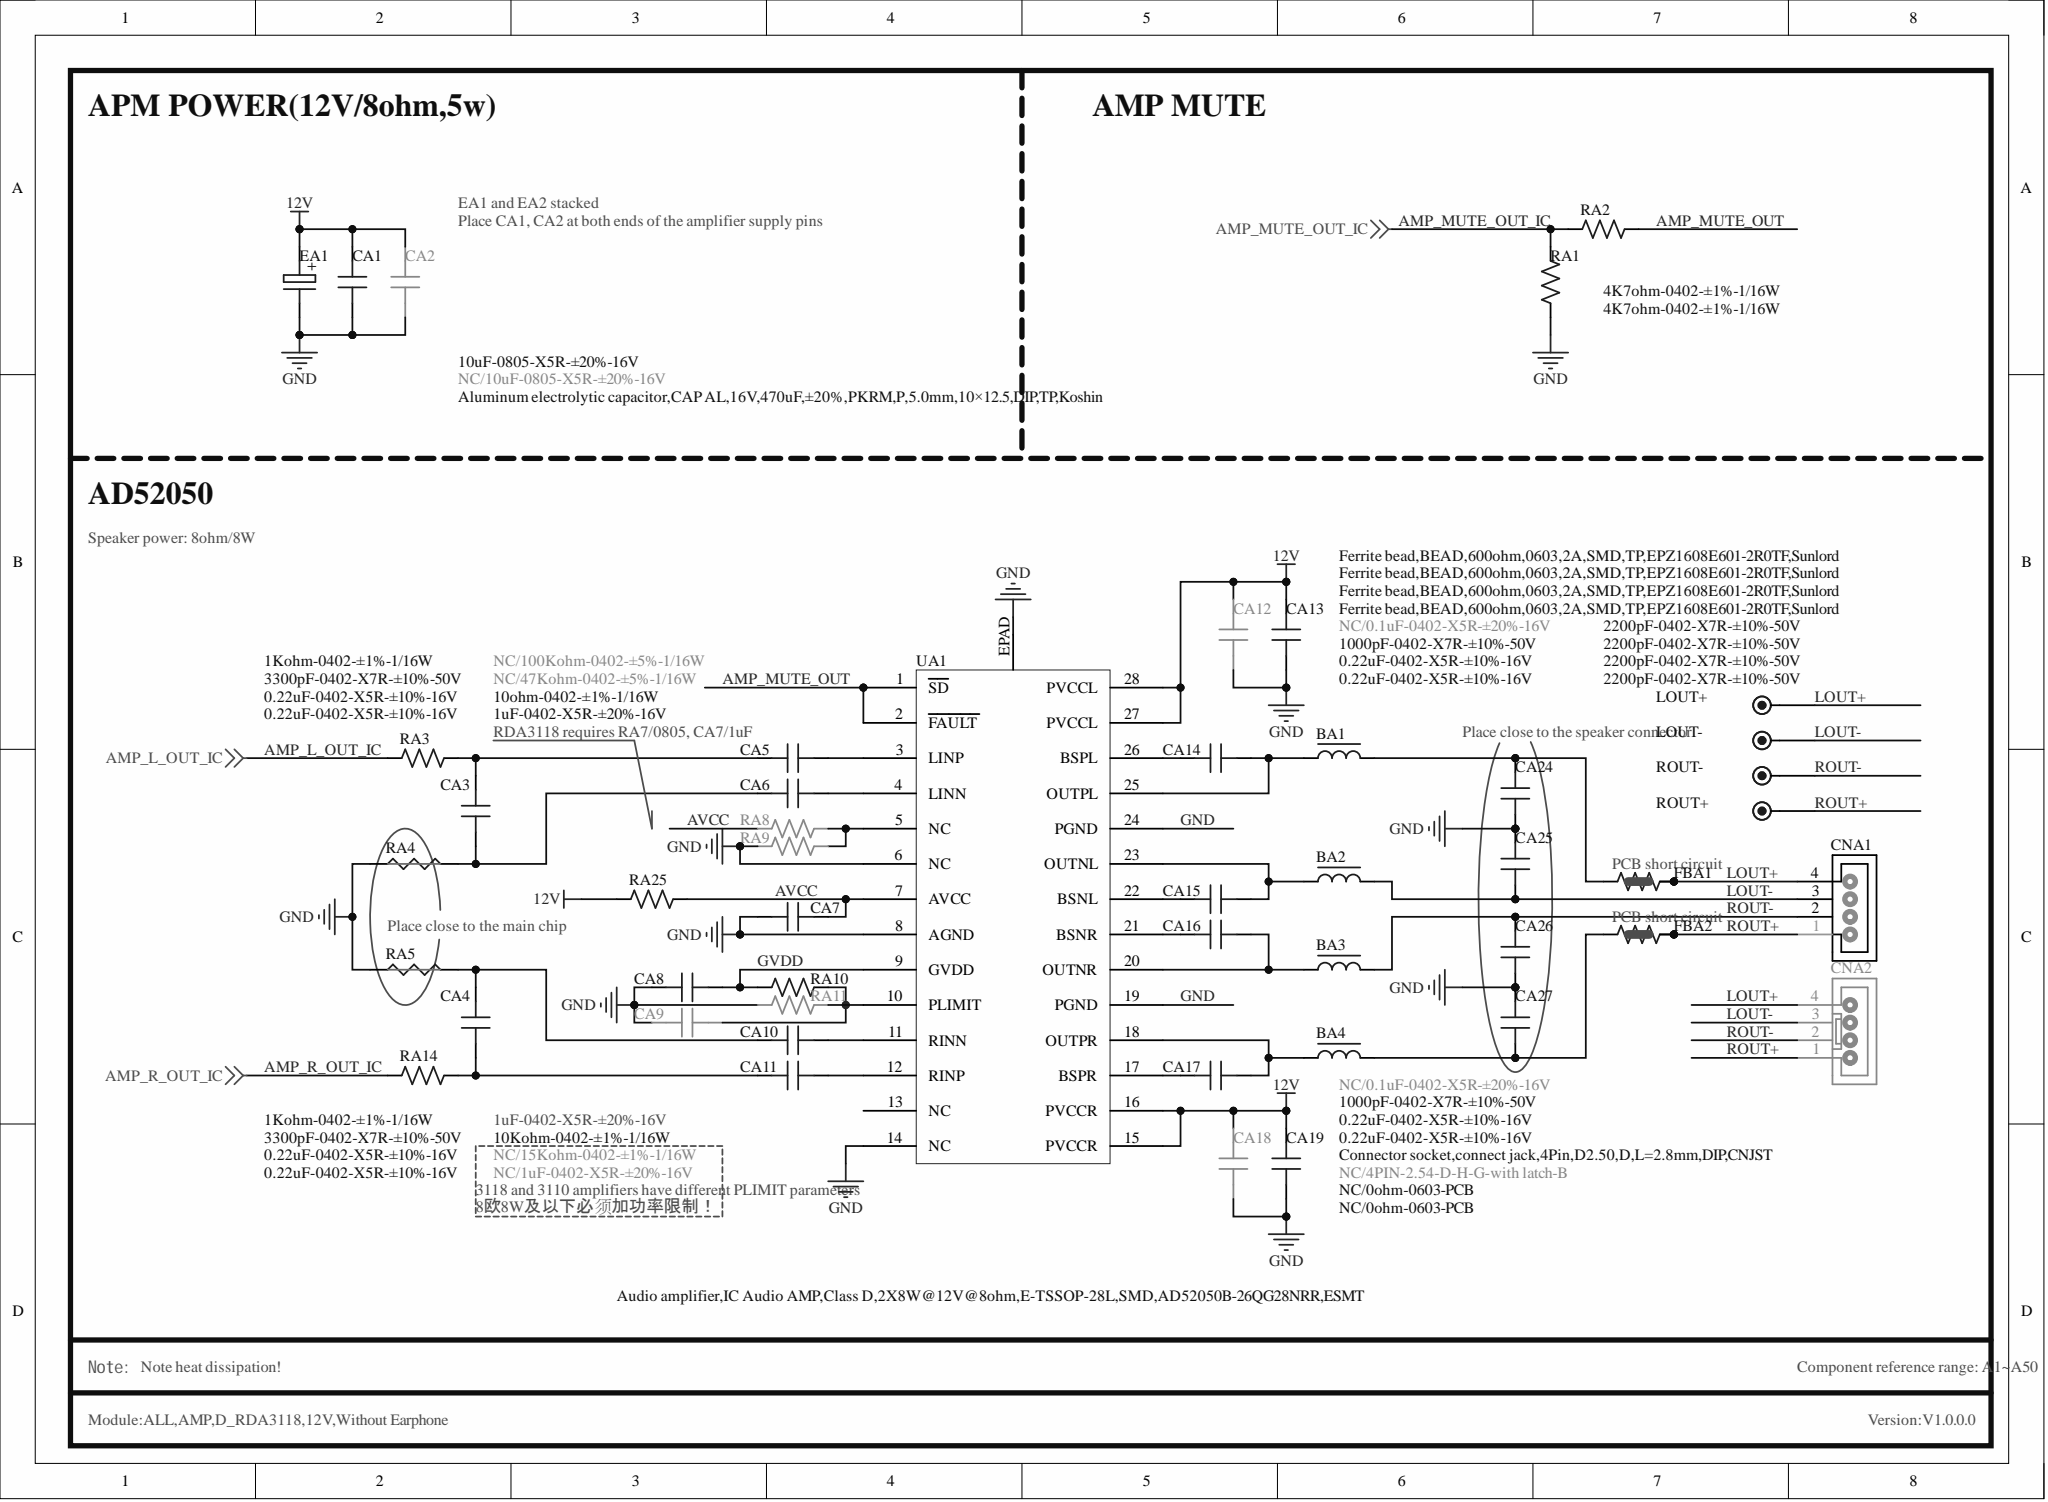Circuit board | Altium Designer | 527 parts | 243 nets | one sheet of the schematic
Parts on this sheet (reference | value | footprint):
BA1 | Ferrite bead,BEAD,600ohm,0603,2A,SMD,TP,EPZ1608E601-2R0TF,Sunlord | L0603
BA2 | Ferrite bead,BEAD,600ohm,0603,2A,SMD,TP,EPZ1608E601-2R0TF,Sunlord | L0603
BA3 | Ferrite bead,BEAD,600ohm,0603,2A,SMD,TP,EPZ1608E601-2R0TF,Sunlord | L0603
BA4 | Ferrite bead,BEAD,600ohm,0603,2A,SMD,TP,EPZ1608E601-2R0TF,Sunlord | L0603
CA1 | 10uF-0805-X5R-±20%-16V | C0805
CA2 | NC/10uF-0805-X5R-±20%-16V | C0805
CA3 | 3300pF-0402-X7R-±10%-50V | C0402
CA4 | 3300pF-0402-X7R-±10%-50V | C0402
CA5 | 0.22uF-0402-X5R-±10%-16V | C0402
CA6 | 0.22uF-0402-X5R-±10%-16V | C0402
CA7 | 1uF-0402-X5R-±20%-16V | C0402
CA8 | 1uF-0402-X5R-±20%-16V | C0402
CA9 | NC/1uF-0402-X5R-±20%-16V | C0402
CA10 | 0.22uF-0402-X5R-±10%-16V | C0402
CA11 | 0.22uF-0402-X5R-±10%-16V | C0402
CA12 | NC/0.1uF-0402-X5R-±20%-16V | C0402
CA13 | 1000pF-0402-X7R-±10%-50V | C0402
CA14 | 0.22uF-0402-X5R-±10%-16V | C0402
CA15 | 0.22uF-0402-X5R-±10%-16V | C0402
CA16 | 0.22uF-0402-X5R-±10%-16V | C0402
CA17 | 0.22uF-0402-X5R-±10%-16V | C0402
CA18 | NC/0.1uF-0402-X5R-±20%-16V | C0402
CA19 | 1000pF-0402-X7R-±10%-50V | C0402
CA24 | 2200pF-0402-X7R-±10%-50V | C0402
CA25 | 2200pF-0402-X7R-±10%-50V | C0402
CA26 | 2200pF-0402-X7R-±10%-50V | C0402
CA27 | 2200pF-0402-X7R-±10%-50V | C0402
CNA1 | Connector socket,connect jack,4Pin,D2.50,D,L=2.8mm,DIP,CNJST | SIP4/2.54D-1
CNA2 | NC/4PIN-2.54-D-H-G-with latch-B | SIP4/2.5D-2
EA1 | Aluminum electrolytic capacitor,CAP AL,16V,470uF,±20%,PKRM,P,5.0mm,10×12.5,DIP,TP,Koshin | EC(10*12)-V-5
FBA1 | NC/0ohm-0603-PCB | R0603SC
FBA2 | NC/0ohm-0603-PCB | R0603SC
LOUT+ | DM0 | TP
LOUT- | DM0 | TP
RA1 | 4K7ohm-0402-±1%-1/16W | R0402
RA2 | 4K7ohm-0402-±1%-1/16W | R0402
RA3 | 1Kohm-0402-±1%-1/16W | R0402
RA4 | NC/? | GND
RA5 | NC/? | GND
RA8 | NC/100Kohm-0402-±5%-1/16W | R0402
RA9 | NC/47Kohm-0402-±5%-1/16W | R0402
RA10 | 10Kohm-0402-±1%-1/16W | R0402
RA11 | NC/15Kohm-0402-±1%-1/16W | R0402
RA14 | 1Kohm-0402-±1%-1/16W | R0402
RA25 | 10ohm-0402-±1%-1/16W | R0402
ROUT+ | DM0 | TP
UA1 | Audio amplifier,IC Audio AMP,Class D,2X8W@12V@8ohm,E-TSSOP-28L,SMD,AD52050B-26QG28NRR,ESMT | SOP28/0.65-7
Nets of these parts (net: part-pin ...):
ROUT-: BA3-2 CA26-2 CNA1-2 CNA2-2
ROUT+: CNA1-1 CNA2-1 FBA2-2 FBA2-3 ROUT+-1
NetRA8_2: RA8-2 RA9-2 UA1-5
NetCA17_1: CA17-1 UA1-17
NetCA16_1: CA16-1 UA1-21
NetCA15_1: CA15-1 UA1-22
NetCA14_1: CA14-1 UA1-26
NetCA11_2: CA11-2 UA1-12
NetCA10_2: CA10-2 UA1-11
NetCA9_2: CA9-2 RA10-2 RA11-2 UA1-10
NetCA6_2: CA6-2 UA1-4
NetCA5_2: CA5-2 UA1-3
NetCA4_2: CA4-2 CA10-1 RA5-JP_1K
NetCA4_1: CA4-1 CA11-1 RA14-2
NetCA3_2: CA3-2 CA5-1 RA3-2
NetCA3_1: CA3-1 CA6-1 RA4-JP_1K
NetBA4_2: BA4-2 CA27-1 FBA2-1
NetBA4_1: BA4-1 CA17-2 UA1-18
NetBA3_1: BA3-1 CA16-2 UA1-20
NetBA2_1: BA2-1 CA15-2 UA1-23
NetBA1_2: BA1-2 CA24-2 FBA1-1
NetBA1_1: BA1-1 CA14-2 UA1-25
LOUT-: BA2-2 CA25-1 CNA1-3 CNA2-3 LOUT--1
LOUT+: CNA1-4 CNA2-4 FBA1-2 FBA1-3 LOUT+-1
GVDD: CA8-2 RA10-1 UA1-9
GND: CA1-1 CA2-1 CA7-1 CA8-1 CA9-1 CA12-1 CA13-1 CA18-1 CA19-1 CA24-1 CA25-2 CA26-1 CA27-2 EA1-2 RA1-2 RA4-JP_2K RA5-JP_2K RA9-1 RA11-1 UA1-6 UA1-8 UA1-14 UA1-19 UA1-24 UA1-EPAD
AVCC: CA7-2 RA8-1 RA25-1 UA1-7
AMP_R_OUT_IC: RA14-1
AMP_MUTE_OUT_IC: RA1-1 RA2-2
AMP_MUTE_OUT: RA2-1 UA1-1 UA1-2
AMP_L_OUT_IC: RA3-1
12V: CA1-2 CA2-2 CA12-2 CA13-2 CA18-2 CA19-2 EA1-1 RA25-2 UA1-15 UA1-16 UA1-27 UA1-28